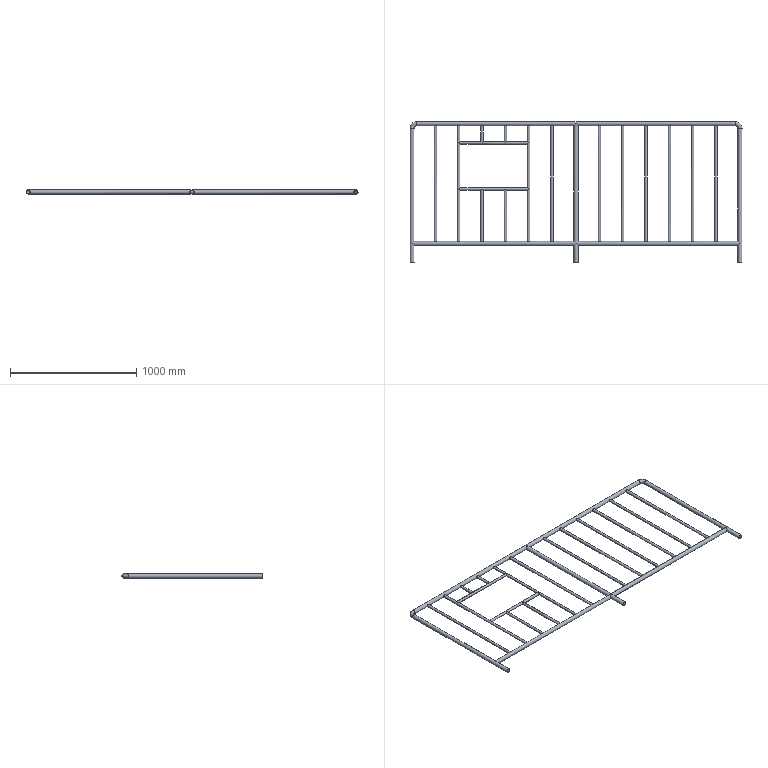Part | STEP file | PN_0056 304 guardrail 2600X1100B_Default<As Machined> | 24 solids | 96 faces | box 2632 x 1116 x 32 mm | volume 2870828 mm3 | cylinder 81 | plane 11 | torus 4 | commonest cylinder face diameters 32 x35 20 x24 16 x16 28 x6